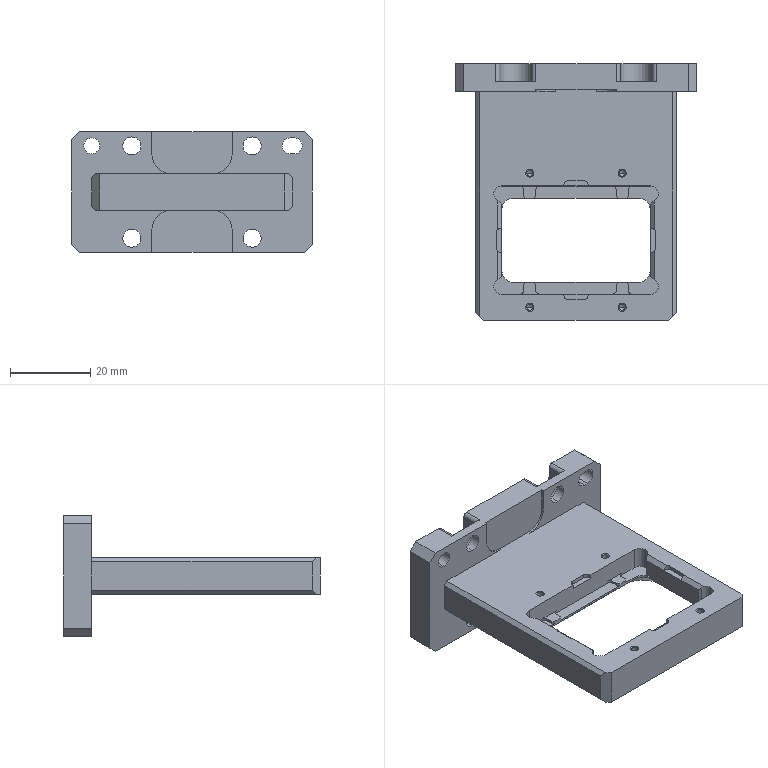NC program | NX | posted with a generic post | part box 60 x 64 x 30 mm
Lines 11437 to 12381 of 12381:
(CAVITY_MILL_COPY_COPY , TOOL : D2)
N22842 T02 M6
N22844 G54
N22846 G17 G0 G90 X25.4 Y0.178 B0. C0. S9500 M3
N22848 G43 Z30. H2
N22850 Z-9.508
N22852 G94 G1 Z-10.508 F1200.
N22854 G3 X25.8 Y0.978 R1.
N22856 G1 Y2.
N22858 X25.72
N22860 X25.5
N22862 G2 X24.924 Y2.182 R1.
N22864 G3 X24.255 Y2.361 R1.
N22866 G1 Z-9.508
N22868 G0 X25.4 Y0.178 Z-9.706
N22870 G1 Z-10.706
N22872 G3 X25.8 Y0.978 R1.
N22874 G1 Y2.
N22876 X25.72
N22878 X25.5
N22880 G2 X24.924 Y2.182 R1.
N22882 G3 X24.255 Y2.361 R1.
N22884 G1 Z-9.706
N22886 G0 X25.4 Y0.178 Z-9.905
N22888 G1 Z-10.905
N22890 G3 X25.8 Y0.978 R1.
N22892 G1 Y2.
N22894 X25.72
N22896 X25.5
N22898 G2 X24.924 Y2.182 R1.
N22900 G3 X24.255 Y2.361 R1.
N22902 G1 Z-9.905
N22904 G0 X25.4 Y0.178 Z-10.103
N22906 G1 Z-11.103
N22908 G3 X25.8 Y0.978 R1.
N22910 G1 Y2.
N22912 X25.72
N22914 X25.5
N22916 G2 X24.924 Y2.182 R1.
N22918 G3 X24.255 Y2.361 R1.
N22920 G1 Z-10.103
N22922 G0 X25.4 Y0.178 Z-10.302
N22924 G1 Z-11.302
N22926 G3 X25.8 Y0.978 R1.
N22928 G1 Y2.
N22930 X25.72
N22932 X25.5
N22934 G2 X24.924 Y2.182 R1.
N22936 G3 X24.255 Y2.361 R1.
N22938 G1 Z-10.302
N22940 G0 X25.4 Y0.178 Z-10.5
N22942 G1 Z-11.5
N22944 G3 X25.8 Y0.978 R1.
N22946 G1 Y1.999
N22948 X25.72 Y2.
N22950 X25.5
N22952 G2 X24.924 Y2.182 R1.
N22954 G3 X24.255 Y2.361 R1.
N22956 G1 Z-10.5
N22958 G0 Z11.
N22960 Y-2.361
N22962 Z-9.508
N22964 G1 Z-10.508
N22966 G3 X24.924 Y-2.182 R1.
N22968 G2 X25.5 Y-2. R1.
N22970 G1 X25.72
N22972 X25.801
N22974 X25.8 Y-1.731
N22976 Y-0.978
N22978 G3 X25.4 Y-0.178 R1.
N22980 G1 Z-9.508
N22982 G0 X24.255 Y-2.361 Z-9.706
N22984 G1 Z-10.706
N22986 G3 X24.924 Y-2.182 R1.
N22988 G2 X25.5 Y-2. R1.
N22990 G1 X25.72
N22992 X25.801 Y-1.999
N22994 X25.8 Y-1.731
N22996 Y-0.978
N22998 G3 X25.4 Y-0.178 R1.
N23000 G1 Z-9.706
N23002 G0 X24.255 Y-2.361 Z-9.905
N23004 G1 Z-10.905
N23006 G3 X24.924 Y-2.182 R1.
N23008 G2 X25.5 Y-2. R1.
N23010 G1 X25.72
N23012 X25.8 Y-1.999
N23014 Y-1.731
N23016 Y-0.978
N23018 G3 X25.328 Y-1.312 R0.5
N23020 X25.272 Y-1.619 R1.
N23022 G1 Z-9.905
N23024 G0 X24.255 Y-2.361 Z-10.103
N23026 G1 Z-11.103
N23028 G3 X24.924 Y-2.182 R1.
N23030 G2 X25.5 Y-2. R1.
N23032 G1 X25.72
N23034 X25.8 Y-1.998
N23036 Y-1.731
N23038 Y-0.978
N23040 G3 X25.328 Y-1.312 R0.5
N23042 X25.272 Y-1.619 R1.
N23044 G1 Z-10.103
N23046 G0 X24.255 Y-2.361 Z-10.302
N23048 G1 Z-11.302
N23050 G3 X24.924 Y-2.182 R1.
N23052 G2 X25.5 Y-2. R1.
N23054 G1 X25.72
N23056 X25.8 Y-1.998
N23058 Y-1.731
N23060 Y-0.978
N23062 G3 X25.4 Y-0.178 R1.
N23064 G1 Z-10.302
N23066 G0 X24.255 Y-2.361 Z-10.5
N23068 G1 Z-11.5
N23070 G3 X24.924 Y-2.182 R1.
N23072 G2 X25.5 Y-2. R1.
N23074 G1 X25.72
N23076 X25.8 Y-1.998
N23078 Y-1.731
N23080 Y-0.978
N23082 G3 X25.4 Y-0.178 R1.
N23084 G1 Z-10.5
N23086 G0 Z-0.31
N23088 X22.599 Y-8.659
N23090 Z-14.6
N23092 G1 Z-15.6
N23094 G3 X23.352 Y-9. R1.
N23096 G1 X24.5
N23098 Y-7.852
N23100 G3 X24.1 Y-7.052 R1.
N23102 G1 Z-14.6
N23104 G0 X22.599 Y-8.659 Z-14.8
N23106 G1 Z-15.8
N23108 G3 X23.352 Y-9. R1.
N23110 G1 X24.5
N23112 Y-7.852
N23114 G3 X24.1 Y-7.052 R1.
N23116 G1 Z-14.8
N23118 G0 X22.599 Y-8.659 Z-15.
N23120 G1 Z-16.
N23122 G3 X23.352 Y-9. R1.
N23124 G1 X24.5
N23126 Y-7.852
N23128 G3 X24.1 Y-7.052 R1.
N23130 G1 Z-15.
N23132 G0 Z-5.4
N23134 Y-15.948
N23136 Z-14.6
N23138 G1 Z-15.6
N23140 G3 X24.5 Y-15.148 R1.
N23142 G1 Y-14.
N23144 X23.352
N23146 G3 X22.599 Y-14.341 R1.
N23148 G1 Z-14.6
N23150 G0 X24.1 Y-15.948 Z-14.8
N23152 G1 Z-15.8
N23154 G3 X24.5 Y-15.148 R1.
N23156 G1 Y-14.
N23158 X23.352
N23160 G3 X22.599 Y-14.341 R1.
N23162 G1 Z-14.8
N23164 G0 X24.1 Y-15.948 Z-15.
N23166 G1 Z-16.
N23168 G3 X24.5 Y-15.148 R1.
N23170 G1 Y-14.
N23172 X23.352
N23174 G3 X22.599 Y-14.341 R1.
N23176 G1 Z-15.
N23178 G0 Z11.
N23180 X12.663 Y-18.4
N23182 Z-9.508
N23184 G1 Z-10.508
N23186 G3 X13.463 Y-18.8 R1.
N23188 G1 X14.
N23190 G2 X14.456 Y-18.528 R0.994
N23192 G3 X15.04 Y-18.092 R1.
N23194 G1 Z-9.508
N23196 G0 X12.263 Y-18.4 Z-9.706
N23198 G1 Z-10.706
N23200 G3 X13.063 Y-18.8 R1.
N23202 G1 X13.996
N23204 G2 X14.642 Y-18.316 R0.975
N23206 G3 X15.26 Y-17.894 R1.
N23208 G1 Z-9.706
N23210 G0 X12.477 Y-18.4 Z-9.905
N23212 G1 Z-10.905
N23214 G3 X13.277 Y-18.8 R1.
N23216 G1 X13.995
N23218 G2 X14.376 Y-18.275 R0.993
N23220 G3 X14.77 Y-17.706 R1.
N23222 G1 Z-9.905
N23224 G0 X12.38 Y-18.4 Z-10.103
N23226 G1 Z-11.103
N23228 G3 X13.18 Y-18.8 R1.
N23230 G1 X13.994
N23232 G2 X14.307 Y-18.166 R1.001
N23234 G3 X14.619 Y-17.547 R1.
N23236 G1 Z-10.103
N23238 G0 X12.264 Y-18.4 Z-10.302
N23240 G1 Z-11.302
N23242 G3 X13.064 Y-18.8 R1.
N23244 G1 X13.993
N23246 G2 X14.245 Y-18.046 R1.024
N23248 G3 X14.494 Y-17.396 R1.
N23250 G1 Z-10.302
N23252 G0 X12.181 Y-18.4 Z-10.5
N23254 G1 Z-11.5
N23256 G3 X12.981 Y-18.8 R1.
N23258 G1 X13.992
N23260 X14.009 Y-18.448
N23262 G2 X14.194 Y-17.917 R0.987
N23264 G3 X14.379 Y-17.251 R1.
N23266 G1 Z-10.5
N23268 G0 Z11.
N23270 X8.959 Y-18.092
N23272 Z-9.508
N23274 G1 Z-10.508
N23276 G3 X9.543 Y-18.528 R1.
N23278 G2 X10. Y-18.8 R0.996
N23280 G1 X10.537
N23282 G3 X11.337 Y-18.4 R1.
N23284 G1 Z-9.508
N23286 G0 X8.933 Y-17.894 Z-9.706
N23288 G1 Z-10.706
N23290 G3 X9.474 Y-18.348 R1.
N23292 G2 X10.002 Y-18.8 R0.962
N23294 G1 X10.83
N23296 G3 X11.63 Y-18.4 R1.
N23298 G1 Z-9.706
N23300 G0 X9.23 Y-17.704 Z-9.905
N23302 G1 Z-10.905
N23304 G3 X9.625 Y-18.27 R1.
N23306 G2 X10.004 Y-18.8 R0.973
N23308 G1 X10.728
N23310 G3 X11.528 Y-18.4 R1.
N23312 G1 Z-9.905
N23314 G0 X9.367 Y-17.542 Z-10.103
N23316 G1 Z-11.103
N23318 G3 X9.686 Y-18.156 R1.
N23320 G2 X10.008 Y-18.8 R0.995
N23322 G1 X10.832
N23324 G3 X11.632 Y-18.4 R1.
N23326 G1 Z-10.103
N23328 G0 X9.506 Y-17.396 Z-10.302
N23330 G1 Z-11.302
N23332 G3 X9.756 Y-18.045 R1.
N23334 G2 X10.009 Y-18.8 R1.023
N23336 G1 X10.939
N23338 G3 X11.739 Y-18.4 R1.
N23340 G1 Z-10.302
N23342 G0 X9.628 Y-17.255 Z-10.5
N23344 G1 Z-11.5
N23346 G3 X9.81 Y-17.922 R1.
N23348 G2 X9.992 Y-18.444 R0.987
N23350 G1 X10.01 Y-18.8
N23352 X11.017
N23354 G3 X11.817 Y-18.4 R1.
N23356 G1 Z-10.5
N23358 G0 Z-1.302
N23360 X1.401 Y-14.341
N23362 Z-14.6
N23364 G1 Z-15.6
N23366 G3 X0.648 Y-14. R1.
N23368 G1 X-0.5
N23370 Y-15.148
N23372 G3 X-0.1 Y-15.948 R1.
N23374 G1 Z-14.6
N23376 G0 X1.401 Y-14.341 Z-14.8
N23378 G1 Z-15.8
N23380 G3 X0.648 Y-14. R1.
N23382 G1 X-0.5
N23384 Y-15.148
N23386 G3 X-0.1 Y-15.948 R1.
N23388 G1 Z-14.8
N23390 G0 X1.401 Y-14.341 Z-15.
N23392 G1 Z-16.
N23394 G3 X0.648 Y-14. R1.
N23396 G1 X-0.5
N23398 Y-15.148
N23400 G3 X-0.1 Y-15.948 R1.
N23402 G1 Z-15.
N23404 G0 Z-5.4
N23406 Y-7.052
N23408 Z-14.6
N23410 G1 Z-15.6
N23412 G3 X-0.5 Y-7.852 R1.
N23414 G1 Y-9.
N23416 X0.648
N23418 G3 X1.401 Y-8.659 R1.
N23420 G1 Z-14.6
N23422 G0 X-0.1 Y-7.052 Z-14.8
N23424 G1 Z-15.8
N23426 G3 X-0.5 Y-7.852 R1.
N23428 G1 Y-9.
N23430 X0.648
N23432 G3 X1.401 Y-8.659 R1.
N23434 G1 Z-14.8
N23436 G0 X-0.1 Y-7.052 Z-15.
N23438 G1 Z-16.
N23440 G3 X-0.5 Y-7.852 R1.
N23442 G1 Y-9.
N23444 X0.648
N23446 G3 X1.401 Y-8.659 R1.
N23448 G1 Z-15.
N23450 G0 Z11.
N23452 X-1.4 Y-0.178
N23454 Z-9.508
N23456 G1 Z-10.508
N23458 G3 X-1.8 Y-0.978 R1.
N23460 G1 Y-2.
N23462 X-1.5
N23464 G2 X-0.924 Y-2.182 R1.
N23466 G3 X-0.255 Y-2.361 R1.
N23468 G1 Z-9.508
N23470 G0 X-1.4 Y-0.178 Z-9.706
N23472 G1 Z-10.706
N23474 G3 X-1.8 Y-0.978 R1.
N23476 G1 Y-2.
N23478 X-1.5
N23480 G2 X-0.924 Y-2.182 R1.
N23482 G3 X-0.255 Y-2.361 R1.
N23484 G1 Z-9.706
N23486 G0 X-1.272 Y-1.619 Z-9.905
N23488 G1 Z-10.905
N23490 G3 X-1.328 Y-1.312 R1.
N23492 X-1.8 Y-0.978 R0.5
N23494 G1 Y-2.
N23496 X-1.5
N23498 G2 X-0.924 Y-2.182 R1.
N23500 G3 X-0.255 Y-2.361 R1.
N23502 G1 Z-9.905
N23504 G0 X-1.4 Y-0.178 Z-10.103
N23506 G1 Z-11.103
N23508 G3 X-1.8 Y-0.978 R1.
N23510 G1 Y-2.
N23512 X-1.5
N23514 G2 X-0.924 Y-2.182 R1.
N23516 G3 X-0.255 Y-2.361 R1.
N23518 G1 Z-10.103
N23520 G0 X-1.4 Y-0.178 Z-10.302
N23522 G1 Z-11.302
N23524 G3 X-1.8 Y-0.978 R1.
N23526 G1 Y-2.
N23528 X-1.5
N23530 G2 X-0.924 Y-2.182 R1.
N23532 G3 X-0.255 Y-2.361 R1.
N23534 G1 Z-10.302
N23536 G0 X-1.4 Y-0.178 Z-10.5
N23538 G1 Z-11.5
N23540 G3 X-1.8 Y-0.978 R1.
N23542 G1 Y-2.
N23544 X-1.5
N23546 G2 X-0.924 Y-2.182 R1.
N23548 G3 X-0.255 Y-2.361 R1.
N23550 G1 Z-10.5
N23552 G0 Z11.
N23554 Y2.361
N23556 Z-9.508
N23558 G1 Z-10.508
N23560 G3 X-0.924 Y2.182 R1.
N23562 G2 X-1.5 Y2. R1.
N23564 G1 X-1.8
N23566 Y0.978
N23568 G3 X-1.328 Y1.312 R0.5
N23570 X-1.272 Y1.619 R1.
N23572 G1 Z-9.508
N23574 G0 X-0.255 Y2.361 Z-9.706
N23576 G1 Z-10.706
N23578 G3 X-0.924 Y2.182 R1.
N23580 G2 X-1.5 Y2. R1.
N23582 G1 X-1.8
N23584 Y0.978
N23586 G3 X-1.328 Y1.312 R0.5
N23588 X-1.272 Y1.619 R1.
N23590 G1 Z-9.706
N23592 G0 X-0.255 Y2.361 Z-9.905
N23594 G1 Z-10.905
N23596 G3 X-0.924 Y2.182 R1.
N23598 G2 X-1.5 Y2. R1.
N23600 G1 X-1.8
N23602 Y0.978
N23604 G3 X-1.328 Y1.312 R0.5
N23606 X-1.272 Y1.619 R1.
N23608 G1 Z-9.905
N23610 G0 X-0.255 Y2.361 Z-10.103
N23612 G1 Z-11.103
N23614 G3 X-0.924 Y2.182 R1.
N23616 G2 X-1.5 Y2. R1.
N23618 G1 X-1.8
N23620 Y0.978
N23622 G3 X-1.4 Y0.178 R1.
N23624 G1 Z-10.103
N23626 G0 X-0.255 Y2.361 Z-10.302
N23628 G1 Z-11.302
N23630 G3 X-0.924 Y2.182 R1.
N23632 G2 X-1.5 Y2. R1.
N23634 G1 X-1.8
N23636 Y0.978
N23638 G3 X-1.4 Y0.178 R1.
N23640 G1 Z-10.302
N23642 G0 X-0.255 Y2.361 Z-10.5
N23644 G1 Z-11.5
N23646 G3 X-0.924 Y2.182 R1.
N23648 G2 X-1.5 Y2. R1.
N23650 G1 X-1.8
N23652 Y0.978
N23654 G3 X-1.4 Y0.178 R1.
N23656 G1 Z-10.5
N23658 G0 Z-0.31
N23660 X1.401 Y8.659
N23662 Z-14.6
N23664 G1 Z-15.6
N23666 G3 X0.648 Y9. R1.
N23668 G1 X-0.5
N23670 Y7.852
N23672 G3 X-0.1 Y7.052 R1.
N23674 G1 Z-14.6
N23676 G0 X1.401 Y8.659 Z-14.8
N23678 G1 Z-15.8
N23680 G3 X0.648 Y9. R1.
N23682 G1 X-0.5
N23684 Y7.852
N23686 G3 X-0.1 Y7.052 R1.
N23688 G1 Z-14.8
N23690 G0 X1.401 Y8.659 Z-15.
N23692 G1 Z-16.
N23694 G3 X0.648 Y9. R1.
N23696 G1 X-0.5
N23698 Y7.852
N23700 G3 X-0.1 Y7.052 R1.
N23702 G1 Z-15.
N23704 G0 Z-5.4
N23706 Y15.948
N23708 Z-14.6
N23710 G1 Z-15.6
N23712 G3 X-0.5 Y15.148 R1.
N23714 G1 Y14.
N23716 X0.648
N23718 G3 X1.401 Y14.341 R1.
N23720 G1 Z-14.6
N23722 G0 X-0.1 Y15.948 Z-14.8
N23724 G1 Z-15.8
N23726 G3 X-0.5 Y15.148 R1.
N23728 G1 Y14.
N23730 X0.648
N23732 G3 X1.401 Y14.341 R1.
N23734 G1 Z-14.8
N23736 G0 X-0.1 Y15.948 Z-15.
N23738 G1 Z-16.
N23740 G3 X-0.5 Y15.148 R1.
N23742 G1 Y14.
N23744 X0.648
N23746 G3 X1.401 Y14.341 R1.
N23748 G1 Z-15.
N23750 G0 Z-0.508
N23752 X11.431 Y18.4
N23754 Z-9.706
N23756 G1 Z-10.706
N23758 G3 X10.631 Y18.8 R1.
N23760 G1 X10.005
N23762 G2 X9.578 Y18.393 R0.977
N23764 G3 X9.1 Y17.894 R1.
N23766 G1 Z-9.706
N23768 G0 X11.525 Y18.4 Z-9.905
N23770 G1 Z-10.905
N23772 G3 X10.725 Y18.8 R1.
N23774 G1 X10.006
N23776 G2 X9.624 Y18.274 R0.993
N23778 G3 X9.229 Y17.706 R1.
N23780 G1 Z-9.905
N23782 G0 X10.266 Y18.277 Z-10.103
N23784 G1 Z-11.103
N23786 G3 X10.491 Y18.328 R1.
N23788 X10.825 Y18.8 R0.5
N23790 G1 X10.007
N23792 G2 X9.686 Y18.161 R1.004
N23794 G3 X9.37 Y17.544 R1.
N23796 G1 Z-10.103
N23798 G0 X10.339 Y18.274 Z-10.302
N23800 G1 Z-11.302
N23802 G3 X10.603 Y18.328 R1.
N23804 X10.937 Y18.8 R0.5
N23806 G1 X10.008
N23808 G2 X9.755 Y18.045 R1.023
N23810 G3 X9.506 Y17.396 R1.
N23812 G1 Z-10.302
N23814 G0 X11.817 Y18.4 Z-10.5
N23816 G1 Z-11.5
N23818 G3 X11.017 Y18.8 R1.
N23820 G1 X10.009
N23822 X10.001 Y18.757
N23824 X9.991 Y18.459
N23826 G2 X9.808 Y17.919 R0.984
N23828 G3 X9.625 Y17.253 R1.
N23830 G1 Z-10.5
N23832 G0 Z-0.508
N23834 X14.902 Y17.894
N23836 Z-9.706
N23838 G1 Z-10.706
N23840 G3 X14.424 Y18.391 R1.
N23842 G2 X13.995 Y18.8 R0.97
N23844 G1 X13.367
N23846 G3 X12.567 Y18.4 R1.
N23848 G1 Z-9.706
N23850 G0 X14.761 Y17.706 Z-9.905
N23852 G1 Z-10.905
N23854 G3 X14.37 Y18.275 R1.
N23856 G2 X13.994 Y18.8 R0.984
N23858 G1 X13.277
N23860 G3 X12.477 Y18.4 R1.
N23862 G1 Z-9.905
N23864 G0 X14.622 Y17.544 Z-10.103
N23866 G1 Z-11.103
N23868 G3 X14.307 Y18.161 R1.
N23870 G2 X13.992 Y18.8 R0.994
N23872 G1 X13.173
N23874 G3 X12.373 Y18.4 R1.
N23876 G1 Z-10.103
N23878 G0 X14.5 Y17.391 Z-10.302
N23880 G1 Z-11.302
N23882 G3 X14.25 Y18.037 R1.
N23884 G2 X14. Y18.698 R1.
N23886 G1 Y18.8
N23888 X13.064
N23890 G3 X13.398 Y18.328 R0.5
N23892 X13.666 Y18.274 R1.
N23894 G1 Z-10.302
N23896 G0 X14.367 Y17.259 Z-10.5
N23898 G1 Z-11.5
N23900 G3 X14.185 Y17.928 R1.
N23902 G2 X14. Y18.507 R1.
N23904 G1 Y18.8
N23906 X12.98
N23908 G3 X13.314 Y18.328 R0.5
N23910 X13.62 Y18.272 R1.
N23912 G1 Z-10.5
N23914 G0 Z-1.103
N23916 X22.599 Y14.341
N23918 Z-14.6
N23920 G1 Z-15.6
N23922 G3 X23.352 Y14. R1.
N23924 G1 X24.5
N23926 Y15.148
N23928 G3 X24.1 Y15.948 R1.
N23930 G1 Z-14.6
N23932 G0 X22.599 Y14.341 Z-14.8
N23934 G1 Z-15.8
N23936 G3 X23.352 Y14. R1.
N23938 G1 X24.5
N23940 Y15.148
N23942 G3 X24.1 Y15.948 R1.
N23944 G1 Z-14.8
N23946 G0 X22.599 Y14.341 Z-15.
N23948 G1 Z-16.
N23950 G3 X23.352 Y14. R1.
N23952 G1 X24.5
N23954 Y15.148
N23956 G3 X24.1 Y15.948 R1.
N23958 G1 Z-15.
N23960 G0 Z-5.4
N23962 Y7.052
N23964 Z-14.6
N23966 G1 Z-15.6
N23968 G3 X24.5 Y7.852 R1.
N23970 G1 Y9.
N23972 X23.352
N23974 G3 X22.599 Y8.659 R1.
N23976 G1 Z-14.6
N23978 G0 X24.1 Y7.052 Z-14.8
N23980 G1 Z-15.8
N23982 G3 X24.5 Y7.852 R1.
N23984 G1 Y8.999
N23986 X23.352 Y9.
N23988 G3 X22.599 Y8.659 R1.
N23990 G1 Z-14.8
N23992 G0 X24.1 Y7.052 Z-15.
N23994 G1 Z-16.
N23996 G3 X24.5 Y7.852 R1.
N23998 G1 Y8.999
N24000 X23.352 Y9.
N24002 G3 X22.599 Y8.659 R1.
N24004 G1 Z-15.
N24006 G0 Z30.
N24008 M5
(ZLEVEL_PROFILE_COPY_1_COPY , TOOL : D4R0.5)
N24010 T05 M6
N24012 G54
N24014 G17 G0 G90 X-22.53 Y8.916 B0. C0. S9500 M3
N24016 G43 Z30. H5
N24018 Z0.8
N24020 G94 G1 Z-0.2 F2500.
N24022 X-23.128 Y8.994
N24024 G3 X-23.497 Y8.84 R0.4
N24026 G1 X-23.5 Y8.678
N24028 Y-7.993
N24030 X-23.499 Y-8.836
N24032 X-23.484 Y-8.764 Z-0.3
N24034 X-23.5 Y-8.694 Z-0.4
N24036 X-23.501 Y-8.678
N24038 Y-8.098
N24040 X-23.5 Y-7.993
N24042 Y8.677
N24044 X-23.461 Y8.722 Z-0.6
N24046 X-23.5 Y8.677
N24048 Y-8.686
N24050 X-23.465 Y-8.718
N24052 Z-0.8
N24054 X-23.5 Y-8.686
N24056 Y8.677
N24058 X-23.461 Y8.722
N24060 Z-1.
N24062 X-23.5 Y8.677
N24064 Y-8.686
N24066 X-23.465 Y-8.718
N24068 Z-1.2
N24070 X-23.495 Y-8.686
N24072 X-23.5 Y-8.677
N24074 Y8.677
N24076 X-23.461 Y8.722
N24078 Z-1.4
N24080 X-23.5 Y8.677
N24082 Y-8.677
N24084 X-23.465 Y-8.718
N24086 Z-1.6
N24088 X-23.5 Y-8.677
N24090 Y8.677
N24092 X-23.461 Y8.722
N24094 Z-1.8
N24096 X-23.5 Y8.677
N24098 Y-8.677
N24100 X-23.465 Y-8.718
N24102 Z-2.
N24104 X-23.5 Y-8.677
N24106 Y8.677
N24108 X-23.461 Y8.722
N24110 Z-2.2
N24112 X-23.5 Y8.677
N24114 Y-8.677
N24116 X-23.465 Y-8.718
N24118 Z-2.4
N24120 X-23.5 Y-8.677
N24122 Y8.677
N24124 X-23.461 Y8.722
N24126 Z-2.6
N24128 X-23.5 Y8.677
N24130 Y-8.677
N24132 X-23.465 Y-8.718
N24134 Z-2.8
N24136 X-23.5 Y-8.677
N24138 Y8.677
N24140 X-23.461 Y8.722
N24142 Z-3.
N24144 X-23.5 Y8.677
N24146 Y-8.677
N24148 X-23.465 Y-8.718
N24150 Z-3.2
N24152 X-23.5 Y-8.677
N24154 Y8.677
N24156 X-23.461 Y8.722
N24158 Z-3.4
N24160 X-23.5 Y8.677
N24162 Y-8.677
N24164 X-23.465 Y-8.718
N24166 Z-3.6
N24168 X-23.5 Y-8.677
N24170 Y8.677
N24172 X-23.461 Y8.722
N24174 X-23.468 Y8.715 Z-3.8
N24176 X-23.5 Y8.677
N24178 Y-8.677
N24180 X-23.465 Y-8.718
N24182 Z-4.
N24184 X-23.5 Y-8.677
N24186 Y8.677
N24188 X-23.468 Y8.715
N24190 Z-4.2
N24192 X-23.5 Y8.677
N24194 Y-8.677
N24196 X-23.465 Y-8.718
N24198 Z-4.4
N24200 X-23.5 Y-8.677
N24202 Y8.677
N24204 X-23.468 Y8.715
N24206 Z-4.6
N24208 X-23.5 Y8.677
N24210 Y-8.677
N24212 X-23.465 Y-8.718
N24214 Z-4.8
N24216 X-23.5 Y-8.677
N24218 Y8.677
N24220 X-23.468 Y8.715
N24222 Z-5.
N24224 X-23.5 Y8.677
N24226 Y-8.677
N24228 X-23.472 Y-8.71
N24230 Z-5.2
N24232 X-23.5 Y-8.677
N24234 Y8.677
N24236 X-23.467 Y8.715
N24238 Z-5.4
N24240 X-23.5 Y8.677
N24242 Y-8.677
N24244 X-23.472 Y-8.71
N24246 Z-5.6
N24248 X-23.5 Y-8.677
N24250 Y8.677
N24252 X-23.467 Y8.715
N24254 Z-5.8
N24256 X-23.5 Y8.677
N24258 Y-8.677
N24260 X-23.471 Y-8.71
N24262 Z-6.
N24264 X-23.5 Y-8.677
N24266 Y8.677
N24268 X-23.467 Y8.715
N24270 X-23.5 Y8.664 Z-6.2
N24272 Y-8.662
N24274 Y-8.654 Z-6.4
N24276 Y8.656
N24278 Y8.64 Z-6.6
N24280 Y-8.636
N24282 Y-8.601 Z-6.8
N24284 Y8.599
N24286 Y8.561 Z-7.
N24288 Y-8.559
N24290 Y-8.515 Z-7.2
N24292 Y8.514
N24294 Y8.45 Z-7.4
N24296 Y-8.45
N24298 Y-8.389 Z-7.6
N24300 Y8.387
N24302 Y8.307 Z-7.8
N24304 Y-8.313
N24306 Y-8.216 Z-8.
N24308 Y8.215
N24310 Y8.11 Z-8.2
N24312 Y-8.109
N24314 Y-8. Z-8.4
N24316 Y8.
N24318 Y7.876 Z-8.6
N24320 Y-7.875
N24322 Y-7.732 Z-8.8
N24324 Y7.734
N24326 Y7.565 Z-9.
N24328 Y-7.565
N24330 Y-7.39 Z-9.2
N24332 Y7.39
N24334 Y7.173 Z-9.4
N24336 Y-7.184
N24338 Y-6.927 Z-9.6
N24340 Y6.927
N24342 Y6.667 Z-9.8
N24344 Y-6.667
N24346 Y-6.375 Z-9.975
N24348 Y6.375
N24350 Y6.037 Z-10.15
N24352 Y-6.037
N24354 Y-5.601 Z-10.325
N24356 Y5.601
N24358 Y4.756 Z-10.5
N24360 Y-4.756
N24362 G3 X-23.186 Y-5.004 R0.4
N24364 G1 X-22.533 Y-5.097
N24366 Z-9.5
N24368 G0 Z30.
N24370 M5
(DRILLING , TOOL : D6A45)
N24372 T07 M6
N24374 G54
N24376 G17 G0 G90 X-4.7 Y11.5 B0. C0. S5000 M3
N24378 G43 Z30. H7
N24380 G94 G81 G98 Z-11.525 F250. R-7.5
N24382 X28.7
N24384 X-4.7 Y-11.5
N24386 X28.7
N24388 G80
N24390 G0 X28.7 Y-11.5 Z30.
(PLANAR_MILL_COPY , TOOL : D6A45)
N24392 X33.85 Y24.27 S9500
N24394 Z-8.25
N24396 G1 Z-11.25 F500.
N24398 X33.15 Y23.866
N24400 G3 X32.65 Y23. R1.
N24402 G1 Y-23. F1250.
N24404 G3 X33.15 Y-23.866 R1.
N24406 G1 X33.85 Y-24.27
N24408 Z-8.25
N24410 G0 Z30.
N24412 X0.35 Y-9.53
N24414 Z-8.25
N24416 G1 Z-11.25 F500.
N24418 X-0.35 Y-9.934
N24420 G3 X-0.85 Y-10.8 R1.
N24422 G1 Y-18.5 F1250.
N24424 G3 X1.664 Y-19.184 R1.35
N24426 G1 X1.787 Y-18.906
N24428 G2 X1.969 Y-18.612 R0.75
N24430 G1 X2.511 Y-18.07
N24432 G2 X3.041 Y-17.85 R0.75
N24434 G1 X8.9
N24436 G2 X9.65 Y-18.6 R0.75
N24438 G1 Y-18.74
N24440 X9.683 Y-18.92
N24442 X9.786 Y-19.077
N24444 G3 X10. Y-19.15 R0.35
N24446 G1 X14.
N24448 G3 X14.214 Y-19.077 R0.35
N24450 G1 X14.317 Y-18.92
N24452 X14.35 Y-18.74
N24454 Y-18.6
N24456 G2 X15.1 Y-17.85 R0.75
N24458 G1 X20.959
N24460 G2 X21.489 Y-18.07 R0.75
N24462 G1 X22.033 Y-18.613
N24464 G2 X22.206 Y-18.884 R0.75
N24466 G1 X22.263 Y-19.037
N24468 X22.339 Y-19.189
N24470 G3 X24.85 Y-18.5 R1.35
N24472 G1 Y-3.1
N24474 G2 X25.6 Y-2.35 R0.75
N24476 G1 X25.8
N24478 G3 X26.15 Y-2. R0.35
N24480 G1 Y2.
N24482 G3 X25.8 Y2.35 R0.35
N24484 G1 X25.6
N24486 G2 X24.85 Y3.1 R0.75
N24488 G1 Y18.5
N24490 G3 X22.339 Y19.189 R1.35
N24492 G1 X22.263 Y19.037
N24494 X22.206 Y18.884
N24496 G2 X22.033 Y18.613 R0.75
N24498 G1 X21.489 Y18.07
N24500 G2 X20.959 Y17.85 R0.75
N24502 G1 X15.1
N24504 G2 X14.35 Y18.6 R0.75
N24506 G1 Y18.74
N24508 X14.317 Y18.92
N24510 X14.214 Y19.077
N24512 G3 X14. Y19.15 R0.35
N24514 G1 X10.
N24516 G3 X9.786 Y19.077 R0.35
N24518 G1 X9.683 Y18.92
N24520 X9.65 Y18.74
N24522 Y18.6
N24524 G2 X8.9 Y17.85 R0.75
N24526 G1 X3.041
N24528 G2 X2.511 Y18.07 R0.75
N24530 G1 X1.967 Y18.613
N24532 G2 X1.794 Y18.884 R0.75
N24534 G1 X1.737 Y19.037
N24536 X1.661 Y19.189
N24538 G3 X-0.85 Y18.5 R1.35
N24540 G1 Y3.1
N24542 G2 X-1.6 Y2.35 R0.75
N24544 G1 X-1.8
N24546 G3 X-2.15 Y2. R0.35
N24548 G1 Y-2.
N24550 G3 X-1.8 Y-2.35 R0.35
N24552 G1 X-1.6
N24554 G2 X-0.85 Y-3.1 R0.75
N24556 G1 Y-10.8
N24558 G3 X-0.35 Y-11.666 R1.
N24560 G1 X0.35 Y-12.07
N24562 Z-8.25
N24564 G0 Z30.
(PLANAR_MILL_COPY_COPY , TOOL : D6A45)
N24566 X32.27 Y-26.7
N24568 Z-9.
N24570 G1 Z-12. F500.
N24572 X31.866 Y-26.
N24574 G3 X31. Y-25.5 R1.
N24576 G1 X-21.5 F1250.
N24578 G3 X-21. Y-26.366 R1.
N24580 G1 X-20.3 Y-26.77
N24582 Z-9.
N24584 G0 Z30.
N24586 Y26.77
N24588 Z-9.
N24590 G1 Z-12. F500.
N24592 X-21. Y26.366
N24594 G3 X-21.5 Y25.5 R1.
N24596 G1 X31. F1250.
N24598 G3 X31.866 Y26. R1.
N24600 G1 X32.27 Y26.7
N24602 Z-9.
N24604 G0 Z30.
(PLANAR_MILL_COPY_COPY_1_COPY , TOOL : D6A45)
N24606 X-33.27 Y31.7
N24608 Z0.5
N24610 G1 Z-2.5 F500.
N24612 X-32.866 Y31.
N24614 G3 X-32. Y30.5 R1.
N24616 G1 X-25. F1250.
N24618 G3 X-24.134 Y31. R1.
N24620 G1 X-23.73 Y31.7
N24622 Z0.5
N24624 G0 Z30.
N24626 Y-31.7
N24628 Z0.5
N24630 G1 Z-2.5 F500.
N24632 X-24.134 Y-31.
N24634 G3 X-25. Y-30.5 R1.
N24636 G1 X-32. F1250.
N24638 G3 X-32.866 Y-31. R1.
N24640 G1 X-33.27 Y-31.7
N24642 Z0.5
N24644 G0 Z30.
(PLANAR_MILL_COPY_COPY_1_COPY_COPY , TOOL : D6A45)
N24646 X23.038 Y16.8
N24648 Z-9.
N24650 G1 Z-12. F500.
N24652 X22.634 Y17.5
N24654 G3 X21.768 Y18. R1.
N24656 G1 X2.232 F1250.
N24658 G3 X1.366 Y17.5 R1.
N24660 G1 X0.962 Y16.8
N24662 Z-9.
N24664 G0 Z30.
N24666 Y-16.8
N24668 Z-9.
N24670 G1 Z-12. F500.
N24672 X1.366 Y-17.5
N24674 G3 X2.232 Y-18. R1.
N24676 G1 X21.768 F1250.
N24678 G3 X22.634 Y-17.5 R1.
N24680 G1 X23.038 Y-16.8
N24682 Z-9.
N24684 G0 Z30.
N24686 M5
N24688 M2